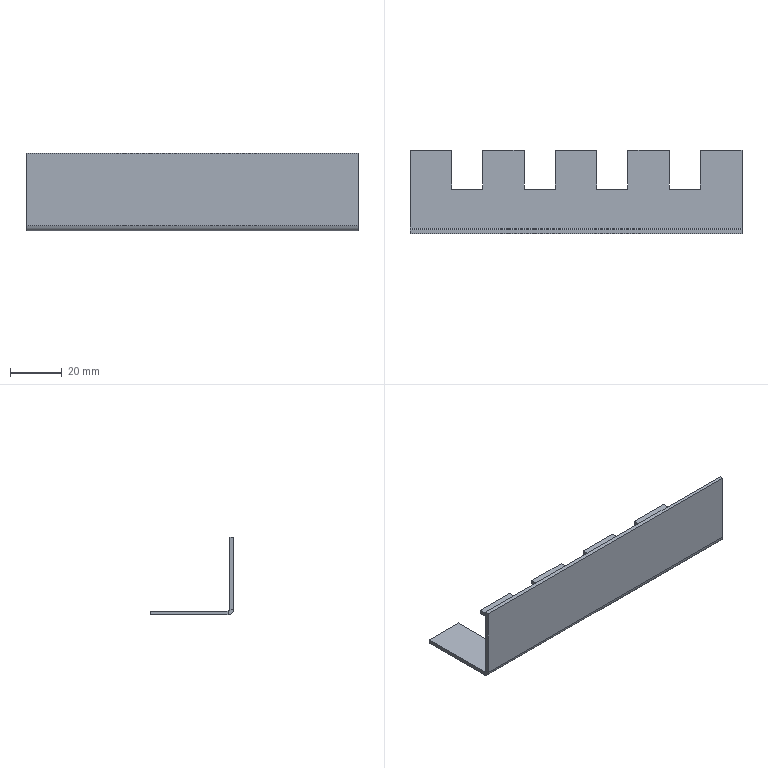Part | STEP file | A14-059 | 1 solid | 30 faces | box 128 x 32.237 x 30 mm | volume 10459 mm3 | plane 28 | cylinder 2 | commonest cylinder face diameters 1.473 x1 4.473 x1